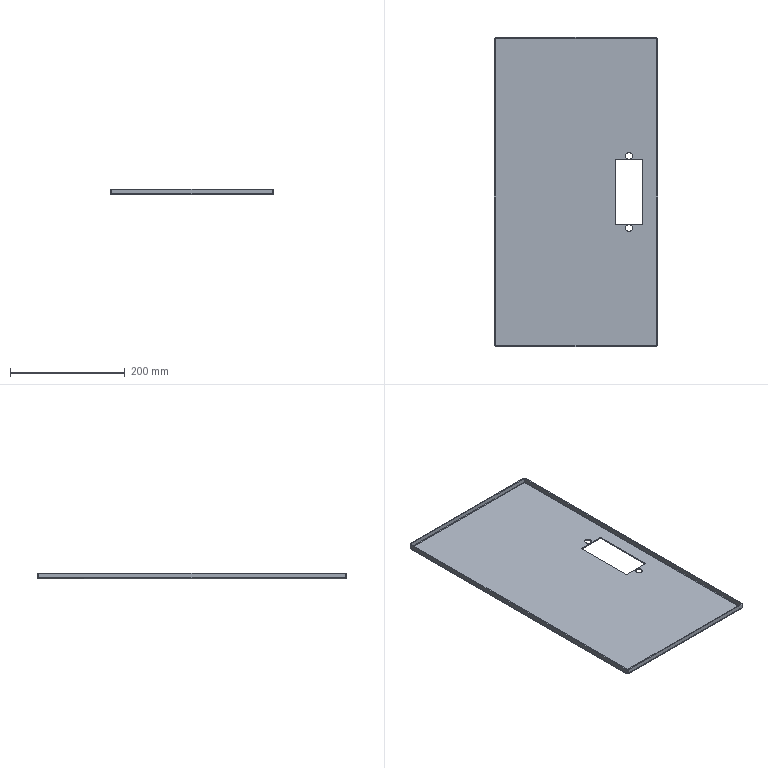Part | SolidWorks | features EdgeFlange 1, FlatPattern 1, ICE 1, SMBaseFlange 1, SheetMetal 1 | 1 solid | 46 faces | box 285 x 540 x 10 mm | volume 320162 mm3 | plane 26 | cylinder 12 | spline 8 | commonest cylinder face diameters 1.473 x4 5.473 x4 12 x4